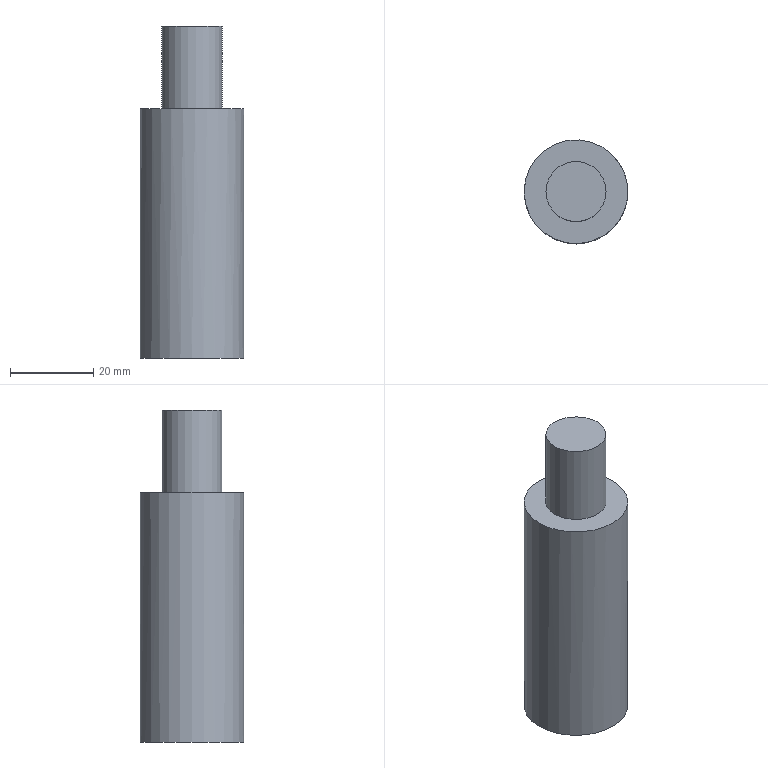Part | NX | features solid 2 | 1 solid | 7 faces | box 25 x 25 x 80 mm | volume 30792 mm3 | plane 4 | cylinder 3 | commonest cylinder face diameters 10 x1 14.5 x1 25 x1
STEP:
#1=CARTESIAN_POINT('',(-572.5,20.,-62.));
#2=VERTEX_POINT('',#1);
#3=CARTESIAN_POINT('',(-560.,20.,-62.));
#4=DIRECTION('',(0.,0.,-1.));
#5=DIRECTION('',(-1.,0.,0.));
#6=AXIS2_PLACEMENT_3D('',#3,#4,#5);
#7=CIRCLE('',#6,12.5);
#8=EDGE_CURVE('',#2,#2,#7,.F.);
#9=ORIENTED_EDGE('',*,*,#8,.F.);
#10=EDGE_LOOP('',(#9));
#11=FACE_BOUND('',#10,.T.);
#12=CARTESIAN_POINT('',(-547.5,20.,-122.));
#13=VERTEX_POINT('',#12);
#14=CARTESIAN_POINT('',(-560.,20.,-122.));
#15=DIRECTION('',(0.,0.,1.));
#16=DIRECTION('',(1.,0.,0.));
#17=AXIS2_PLACEMENT_3D('',#14,#15,#16);
#18=CIRCLE('',#17,12.5);
#19=EDGE_CURVE('',#13,#13,#18,.T.);
#20=ORIENTED_EDGE('',*,*,#19,.T.);
#21=EDGE_LOOP('',(#20));
#22=FACE_BOUND('',#21,.T.);
#23=CARTESIAN_POINT('',(-560.,20.,-22.));
#24=DIRECTION('',(0.,0.,-1.));
#25=DIRECTION('',(-1.,0.,0.));
#26=AXIS2_PLACEMENT_3D('',#23,#24,#25);
#27=CYLINDRICAL_SURFACE('',#26,12.5);
#28=ADVANCED_FACE('',(#11,#22),#27,.T.);
#29=CARTESIAN_POINT('',(-555.,20.,-122.));
#30=VERTEX_POINT('',#29);
#31=CARTESIAN_POINT('',(-560.,20.,-122.));
#32=DIRECTION('',(0.,0.,1.));
#33=DIRECTION('',(1.,0.,0.));
#34=AXIS2_PLACEMENT_3D('',#31,#32,#33);
#35=CIRCLE('',#34,5.);
#36=EDGE_CURVE('',#30,#30,#35,.T.);
#37=ORIENTED_EDGE('',*,*,#36,.T.);
#38=EDGE_LOOP('',(#37));
#39=FACE_BOUND('',#38,.T.);
#40=ORIENTED_EDGE('',*,*,#19,.F.);
#41=EDGE_LOOP('',(#40));
#42=FACE_BOUND('',#41,.T.);
#43=CARTESIAN_POINT('',(-560.,20.,-122.));
#44=DIRECTION('',(0.,0.,1.));
#45=DIRECTION('',(1.,0.,0.));
#46=AXIS2_PLACEMENT_3D('',#43,#44,#45);
#47=PLANE('',#46);
#48=ADVANCED_FACE('',(#39,#42),#47,.F.);
#49=ORIENTED_EDGE('',*,*,#36,.F.);
#50=EDGE_LOOP('',(#49));
#51=FACE_BOUND('',#50,.T.);
#52=CARTESIAN_POINT('',(-555.,20.,-97.));
#53=VERTEX_POINT('',#52);
#54=CARTESIAN_POINT('',(-560.,20.,-97.));
#55=DIRECTION('',(0.,0.,1.));
#56=DIRECTION('',(1.,0.,0.));
#57=AXIS2_PLACEMENT_3D('',#54,#55,#56);
#58=CIRCLE('',#57,5.);
#59=EDGE_CURVE('',#53,#53,#58,.T.);
#60=ORIENTED_EDGE('',*,*,#59,.T.);
#61=EDGE_LOOP('',(#60));
#62=FACE_BOUND('',#61,.T.);
#63=CARTESIAN_POINT('',(-560.,20.,-122.));
#64=DIRECTION('',(0.,0.,1.));
#65=DIRECTION('',(1.,0.,0.));
#66=AXIS2_PLACEMENT_3D('',#63,#64,#65);
#67=CYLINDRICAL_SURFACE('',#66,5.);
#68=ADVANCED_FACE('',(#51,#62),#67,.F.);
#69=ORIENTED_EDGE('',*,*,#59,.F.);
#70=EDGE_LOOP('',(#69));
#71=FACE_BOUND('',#70,.T.);
#72=CARTESIAN_POINT('',(-560.,20.,-97.));
#73=DIRECTION('',(0.,0.,1.));
#74=DIRECTION('',(1.,0.,0.));
#75=AXIS2_PLACEMENT_3D('',#72,#73,#74);
#76=PLANE('',#75);
#77=ADVANCED_FACE('',(#71),#76,.F.);
#78=CARTESIAN_POINT('',(-552.75,20.,-42.));
#79=VERTEX_POINT('',#78);
#80=CARTESIAN_POINT('',(-560.,20.,-42.));
#81=DIRECTION('',(0.,0.,1.));
#82=DIRECTION('',(1.,0.,0.));
#83=AXIS2_PLACEMENT_3D('',#80,#81,#82);
#84=CIRCLE('',#83,7.25);
#85=EDGE_CURVE('',#79,#79,#84,.T.);
#86=ORIENTED_EDGE('',*,*,#85,.F.);
#87=EDGE_LOOP('',(#86));
#88=FACE_BOUND('',#87,.T.);
#89=CARTESIAN_POINT('',(-567.25,20.,-62.));
#90=VERTEX_POINT('',#89);
#91=CARTESIAN_POINT('',(-560.,20.,-62.));
#92=DIRECTION('',(0.,0.,-1.));
#93=DIRECTION('',(-1.,0.,0.));
#94=AXIS2_PLACEMENT_3D('',#91,#92,#93);
#95=CIRCLE('',#94,7.25);
#96=EDGE_CURVE('',#90,#90,#95,.F.);
#97=ORIENTED_EDGE('',*,*,#96,.T.);
#98=EDGE_LOOP('',(#97));
#99=FACE_BOUND('',#98,.T.);
#100=CARTESIAN_POINT('',(-560.,20.,-62.));
#101=DIRECTION('',(0.,0.,1.));
#102=DIRECTION('',(1.,0.,0.));
#103=AXIS2_PLACEMENT_3D('',#100,#101,#102);
#104=CYLINDRICAL_SURFACE('',#103,7.25);
#105=ADVANCED_FACE('',(#88,#99),#104,.T.);
#106=ORIENTED_EDGE('',*,*,#96,.F.);
#107=EDGE_LOOP('',(#106));
#108=FACE_BOUND('',#107,.T.);
#109=ORIENTED_EDGE('',*,*,#8,.T.);
#110=EDGE_LOOP('',(#109));
#111=FACE_BOUND('',#110,.T.);
#112=CARTESIAN_POINT('',(-560.,20.,-62.));
#113=DIRECTION('',(0.,0.,-1.));
#114=DIRECTION('',(-1.,0.,0.));
#115=AXIS2_PLACEMENT_3D('',#112,#113,#114);
#116=PLANE('',#115);
#117=ADVANCED_FACE('',(#108,#111),#116,.F.);
#118=ORIENTED_EDGE('',*,*,#85,.T.);
#119=EDGE_LOOP('',(#118));
#120=FACE_BOUND('',#119,.T.);
#121=CARTESIAN_POINT('',(-560.,20.,-42.));
#122=DIRECTION('',(0.,0.,1.));
#123=DIRECTION('',(1.,0.,0.));
#124=AXIS2_PLACEMENT_3D('',#121,#122,#123);
#125=PLANE('',#124);
#126=ADVANCED_FACE('',(#120),#125,.T.);
#127=CLOSED_SHELL('',(#28,#48,#68,#77,#105,#117,#126));
#128=MANIFOLD_SOLID_BREP('',#127);
#129=(LENGTH_UNIT()NAMED_UNIT(*)SI_UNIT(.MILLI.,.METRE.));
#130=UNCERTAINTY_MEASURE_WITH_UNIT(LENGTH_MEASURE(0.00001),#129,'','');
#131=(NAMED_UNIT(*)PLANE_ANGLE_UNIT()SI_UNIT($,.RADIAN.));
#132=(NAMED_UNIT(*)SI_UNIT($,.STERADIAN.)SOLID_ANGLE_UNIT());
#133=(GEOMETRIC_REPRESENTATION_CONTEXT(3)GLOBAL_UNCERTAINTY_ASSIGNED_CONTEXT((#130))GLOBAL_UNIT_ASSIGNED_CONTEXT((#129,#131,#132))REPRESENTATION_CONTEXT('',''));
#134=ADVANCED_BREP_SHAPE_REPRESENTATION('',(#128),#133);